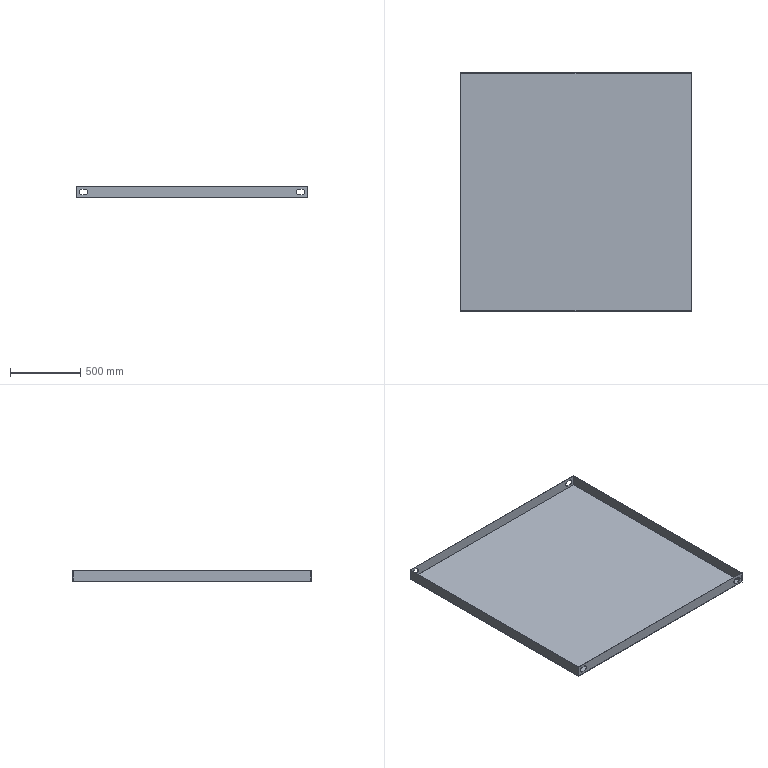Part | SolidWorks | features Extrusion 1, ICE 1, Shell 1 | 1 solid | 27 faces | box 1650 x 1700 x 80 mm | volume 7628292 mm3 | plane 19 | cylinder 8 | commonest cylinder face diameters 40 x8
STEP:
#1=CARTESIAN_POINT('',(825.,-850.,0.));
#2=VERTEX_POINT('',#1);
#3=CARTESIAN_POINT('',(825.,850.,0.));
#4=VERTEX_POINT('',#3);
#5=CARTESIAN_POINT('',(825.,850.,0.));
#6=DIRECTION('',(0.,1.,0.));
#7=VECTOR('',#6,1000.);
#8=LINE('',#5,#7);
#9=EDGE_CURVE('',#2,#4,#8,.T.);
#10=ORIENTED_EDGE('',*,*,#9,.T.);
#11=CARTESIAN_POINT('',(825.,850.,80.));
#12=VERTEX_POINT('',#11);
#13=CARTESIAN_POINT('',(825.,850.,80.));
#14=DIRECTION('',(0.,0.,-1.));
#15=VECTOR('',#14,1000.);
#16=LINE('',#13,#15);
#17=EDGE_CURVE('',#12,#4,#16,.T.);
#18=ORIENTED_EDGE('',*,*,#17,.F.);
#19=CARTESIAN_POINT('',(825.,-850.,80.));
#20=VERTEX_POINT('',#19);
#21=CARTESIAN_POINT('',(825.,850.,80.));
#22=DIRECTION('',(0.,1.,0.));
#23=VECTOR('',#22,1000.);
#24=LINE('',#21,#23);
#25=EDGE_CURVE('',#20,#12,#24,.T.);
#26=ORIENTED_EDGE('',*,*,#25,.F.);
#27=CARTESIAN_POINT('',(825.,-850.,80.));
#28=DIRECTION('',(0.,0.,-1.));
#29=VECTOR('',#28,1000.);
#30=LINE('',#27,#29);
#31=EDGE_CURVE('',#20,#2,#30,.T.);
#32=ORIENTED_EDGE('',*,*,#31,.T.);
#33=EDGE_LOOP('',(#10,#18,#26,#32));
#34=FACE_OUTER_BOUND('',#33,.T.);
#35=CARTESIAN_POINT('',(825.,850.,80.));
#36=DIRECTION('',(-1.,0.,0.));
#37=DIRECTION('',(0.,-1.,0.));
#38=AXIS2_PLACEMENT_3D('',#35,#36,#37);
#39=PLANE('',#38);
#40=ADVANCED_FACE('',(#34),#39,.F.);
#41=CARTESIAN_POINT('',(-765.,850.,60.));
#42=VERTEX_POINT('',#41);
#43=CARTESIAN_POINT('',(-785.,850.,60.));
#44=VERTEX_POINT('',#43);
#45=CARTESIAN_POINT('',(-785.,850.,60.));
#46=DIRECTION('',(-1.,0.,0.));
#47=VECTOR('',#46,1000.);
#48=LINE('',#45,#47);
#49=EDGE_CURVE('',#42,#44,#48,.T.);
#50=ORIENTED_EDGE('',*,*,#49,.T.);
#51=CARTESIAN_POINT('',(-785.,850.,20.));
#52=VERTEX_POINT('',#51);
#53=CARTESIAN_POINT('',(-785.,850.,40.));
#54=DIRECTION('',(0.,-1.,0.));
#55=DIRECTION('',(0.,0.,-1.));
#56=AXIS2_PLACEMENT_3D('',#53,#54,#55);
#57=CIRCLE('',#56,20.);
#58=EDGE_CURVE('',#44,#52,#57,.T.);
#59=ORIENTED_EDGE('',*,*,#58,.T.);
#60=CARTESIAN_POINT('',(-765.,850.,20.));
#61=VERTEX_POINT('',#60);
#62=CARTESIAN_POINT('',(-785.,850.,20.));
#63=DIRECTION('',(1.,0.,0.));
#64=VECTOR('',#63,1000.);
#65=LINE('',#62,#64);
#66=EDGE_CURVE('',#52,#61,#65,.T.);
#67=ORIENTED_EDGE('',*,*,#66,.T.);
#68=CARTESIAN_POINT('',(-765.,850.,40.));
#69=DIRECTION('',(0.,-1.,0.));
#70=DIRECTION('',(0.,0.,-1.));
#71=AXIS2_PLACEMENT_3D('',#68,#69,#70);
#72=CIRCLE('',#71,20.);
#73=EDGE_CURVE('',#61,#42,#72,.T.);
#74=ORIENTED_EDGE('',*,*,#73,.T.);
#75=EDGE_LOOP('',(#50,#59,#67,#74));
#76=FACE_BOUND('',#75,.T.);
#77=CARTESIAN_POINT('',(765.,850.,20.));
#78=VERTEX_POINT('',#77);
#79=CARTESIAN_POINT('',(785.,850.,20.));
#80=VERTEX_POINT('',#79);
#81=CARTESIAN_POINT('',(785.,850.,20.));
#82=DIRECTION('',(1.,0.,0.));
#83=VECTOR('',#82,1000.);
#84=LINE('',#81,#83);
#85=EDGE_CURVE('',#78,#80,#84,.T.);
#86=ORIENTED_EDGE('',*,*,#85,.T.);
#87=CARTESIAN_POINT('',(785.,850.,60.));
#88=VERTEX_POINT('',#87);
#89=CARTESIAN_POINT('',(785.,850.,40.));
#90=DIRECTION('',(0.,-1.,0.));
#91=DIRECTION('',(0.,0.,1.));
#92=AXIS2_PLACEMENT_3D('',#89,#90,#91);
#93=CIRCLE('',#92,20.);
#94=EDGE_CURVE('',#80,#88,#93,.T.);
#95=ORIENTED_EDGE('',*,*,#94,.T.);
#96=CARTESIAN_POINT('',(765.,850.,60.));
#97=VERTEX_POINT('',#96);
#98=CARTESIAN_POINT('',(785.,850.,60.));
#99=DIRECTION('',(-1.,0.,0.));
#100=VECTOR('',#99,1000.);
#101=LINE('',#98,#100);
#102=EDGE_CURVE('',#88,#97,#101,.T.);
#103=ORIENTED_EDGE('',*,*,#102,.T.);
#104=CARTESIAN_POINT('',(765.,850.,40.));
#105=DIRECTION('',(0.,-1.,0.));
#106=DIRECTION('',(0.,0.,1.));
#107=AXIS2_PLACEMENT_3D('',#104,#105,#106);
#108=CIRCLE('',#107,20.);
#109=EDGE_CURVE('',#97,#78,#108,.T.);
#110=ORIENTED_EDGE('',*,*,#109,.T.);
#111=EDGE_LOOP('',(#86,#95,#103,#110));
#112=FACE_BOUND('',#111,.T.);
#113=CARTESIAN_POINT('',(-825.,850.,0.));
#114=VERTEX_POINT('',#113);
#115=CARTESIAN_POINT('',(-825.,850.,0.));
#116=DIRECTION('',(-1.,0.,0.));
#117=VECTOR('',#116,1000.);
#118=LINE('',#115,#117);
#119=EDGE_CURVE('',#4,#114,#118,.T.);
#120=ORIENTED_EDGE('',*,*,#119,.T.);
#121=CARTESIAN_POINT('',(-825.,850.,80.));
#122=VERTEX_POINT('',#121);
#123=CARTESIAN_POINT('',(-825.,850.,80.));
#124=DIRECTION('',(0.,0.,-1.));
#125=VECTOR('',#124,1000.);
#126=LINE('',#123,#125);
#127=EDGE_CURVE('',#122,#114,#126,.T.);
#128=ORIENTED_EDGE('',*,*,#127,.F.);
#129=CARTESIAN_POINT('',(-825.,850.,80.));
#130=DIRECTION('',(-1.,0.,0.));
#131=VECTOR('',#130,1000.);
#132=LINE('',#129,#131);
#133=EDGE_CURVE('',#12,#122,#132,.T.);
#134=ORIENTED_EDGE('',*,*,#133,.F.);
#135=ORIENTED_EDGE('',*,*,#17,.T.);
#136=EDGE_LOOP('',(#120,#128,#134,#135));
#137=FACE_OUTER_BOUND('',#136,.T.);
#138=CARTESIAN_POINT('',(-825.,850.,80.));
#139=DIRECTION('',(0.,-1.,0.));
#140=DIRECTION('',(0.,0.,-1.));
#141=AXIS2_PLACEMENT_3D('',#138,#139,#140);
#142=PLANE('',#141);
#143=ADVANCED_FACE('',(#76,#112,#137),#142,.F.);
#144=CARTESIAN_POINT('',(-825.,-850.,0.));
#145=VERTEX_POINT('',#144);
#146=CARTESIAN_POINT('',(-825.,850.,0.));
#147=DIRECTION('',(0.,-1.,0.));
#148=VECTOR('',#147,1000.);
#149=LINE('',#146,#148);
#150=EDGE_CURVE('',#114,#145,#149,.T.);
#151=ORIENTED_EDGE('',*,*,#150,.T.);
#152=CARTESIAN_POINT('',(-825.,-850.,80.));
#153=VERTEX_POINT('',#152);
#154=CARTESIAN_POINT('',(-825.,-850.,80.));
#155=DIRECTION('',(0.,0.,-1.));
#156=VECTOR('',#155,1000.);
#157=LINE('',#154,#156);
#158=EDGE_CURVE('',#153,#145,#157,.T.);
#159=ORIENTED_EDGE('',*,*,#158,.F.);
#160=CARTESIAN_POINT('',(-825.,850.,80.));
#161=DIRECTION('',(0.,-1.,0.));
#162=VECTOR('',#161,1000.);
#163=LINE('',#160,#162);
#164=EDGE_CURVE('',#122,#153,#163,.T.);
#165=ORIENTED_EDGE('',*,*,#164,.F.);
#166=ORIENTED_EDGE('',*,*,#127,.T.);
#167=EDGE_LOOP('',(#151,#159,#165,#166));
#168=FACE_OUTER_BOUND('',#167,.T.);
#169=CARTESIAN_POINT('',(-825.,850.,80.));
#170=DIRECTION('',(1.,0.,0.));
#171=DIRECTION('',(0.,1.,0.));
#172=AXIS2_PLACEMENT_3D('',#169,#170,#171);
#173=PLANE('',#172);
#174=ADVANCED_FACE('',(#168),#173,.F.);
#175=CARTESIAN_POINT('',(-785.,-850.,20.));
#176=VERTEX_POINT('',#175);
#177=CARTESIAN_POINT('',(-765.,-850.,20.));
#178=VERTEX_POINT('',#177);
#179=CARTESIAN_POINT('',(-785.,-850.,20.));
#180=DIRECTION('',(1.,0.,0.));
#181=VECTOR('',#180,1000.);
#182=LINE('',#179,#181);
#183=EDGE_CURVE('',#176,#178,#182,.T.);
#184=ORIENTED_EDGE('',*,*,#183,.F.);
#185=CARTESIAN_POINT('',(-785.,-850.,60.));
#186=VERTEX_POINT('',#185);
#187=CARTESIAN_POINT('',(-785.,-850.,40.));
#188=DIRECTION('',(0.,-1.,0.));
#189=DIRECTION('',(0.,0.,-1.));
#190=AXIS2_PLACEMENT_3D('',#187,#188,#189);
#191=CIRCLE('',#190,20.);
#192=EDGE_CURVE('',#186,#176,#191,.T.);
#193=ORIENTED_EDGE('',*,*,#192,.F.);
#194=CARTESIAN_POINT('',(-765.,-850.,60.));
#195=VERTEX_POINT('',#194);
#196=CARTESIAN_POINT('',(-785.,-850.,60.));
#197=DIRECTION('',(-1.,0.,0.));
#198=VECTOR('',#197,1000.);
#199=LINE('',#196,#198);
#200=EDGE_CURVE('',#195,#186,#199,.T.);
#201=ORIENTED_EDGE('',*,*,#200,.F.);
#202=CARTESIAN_POINT('',(-765.,-850.,40.));
#203=DIRECTION('',(0.,-1.,0.));
#204=DIRECTION('',(0.,0.,-1.));
#205=AXIS2_PLACEMENT_3D('',#202,#203,#204);
#206=CIRCLE('',#205,20.);
#207=EDGE_CURVE('',#178,#195,#206,.T.);
#208=ORIENTED_EDGE('',*,*,#207,.F.);
#209=EDGE_LOOP('',(#184,#193,#201,#208));
#210=FACE_BOUND('',#209,.T.);
#211=CARTESIAN_POINT('',(785.,-850.,60.));
#212=VERTEX_POINT('',#211);
#213=CARTESIAN_POINT('',(765.,-850.,60.));
#214=VERTEX_POINT('',#213);
#215=CARTESIAN_POINT('',(785.,-850.,60.));
#216=DIRECTION('',(-1.,0.,0.));
#217=VECTOR('',#216,1000.);
#218=LINE('',#215,#217);
#219=EDGE_CURVE('',#212,#214,#218,.T.);
#220=ORIENTED_EDGE('',*,*,#219,.F.);
#221=CARTESIAN_POINT('',(785.,-850.,20.));
#222=VERTEX_POINT('',#221);
#223=CARTESIAN_POINT('',(785.,-850.,40.));
#224=DIRECTION('',(0.,-1.,0.));
#225=DIRECTION('',(0.,0.,1.));
#226=AXIS2_PLACEMENT_3D('',#223,#224,#225);
#227=CIRCLE('',#226,20.);
#228=EDGE_CURVE('',#222,#212,#227,.T.);
#229=ORIENTED_EDGE('',*,*,#228,.F.);
#230=CARTESIAN_POINT('',(765.,-850.,20.));
#231=VERTEX_POINT('',#230);
#232=CARTESIAN_POINT('',(785.,-850.,20.));
#233=DIRECTION('',(1.,0.,0.));
#234=VECTOR('',#233,1000.);
#235=LINE('',#232,#234);
#236=EDGE_CURVE('',#231,#222,#235,.T.);
#237=ORIENTED_EDGE('',*,*,#236,.F.);
#238=CARTESIAN_POINT('',(765.,-850.,40.));
#239=DIRECTION('',(0.,-1.,0.));
#240=DIRECTION('',(0.,0.,1.));
#241=AXIS2_PLACEMENT_3D('',#238,#239,#240);
#242=CIRCLE('',#241,20.);
#243=EDGE_CURVE('',#214,#231,#242,.T.);
#244=ORIENTED_EDGE('',*,*,#243,.F.);
#245=EDGE_LOOP('',(#220,#229,#237,#244));
#246=FACE_BOUND('',#245,.T.);
#247=CARTESIAN_POINT('',(-825.,-850.,0.));
#248=DIRECTION('',(1.,0.,0.));
#249=VECTOR('',#248,1000.);
#250=LINE('',#247,#249);
#251=EDGE_CURVE('',#145,#2,#250,.T.);
#252=ORIENTED_EDGE('',*,*,#251,.T.);
#253=ORIENTED_EDGE('',*,*,#31,.F.);
#254=CARTESIAN_POINT('',(-825.,-850.,80.));
#255=DIRECTION('',(1.,0.,0.));
#256=VECTOR('',#255,1000.);
#257=LINE('',#254,#256);
#258=EDGE_CURVE('',#153,#20,#257,.T.);
#259=ORIENTED_EDGE('',*,*,#258,.F.);
#260=ORIENTED_EDGE('',*,*,#158,.T.);
#261=EDGE_LOOP('',(#252,#253,#259,#260));
#262=FACE_OUTER_BOUND('',#261,.T.);
#263=CARTESIAN_POINT('',(-825.,-850.,80.));
#264=DIRECTION('',(0.,1.,0.));
#265=DIRECTION('',(0.,0.,1.));
#266=AXIS2_PLACEMENT_3D('',#263,#264,#265);
#267=PLANE('',#266);
#268=ADVANCED_FACE('',(#210,#246,#262),#267,.F.);
#269=CARTESIAN_POINT('',(822.7,-847.7,80.));
#270=VERTEX_POINT('',#269);
#271=CARTESIAN_POINT('',(822.7,847.7,80.));
#272=VERTEX_POINT('',#271);
#273=CARTESIAN_POINT('',(822.7,850.,80.));
#274=DIRECTION('',(0.,1.,0.));
#275=VECTOR('',#274,1000.);
#276=LINE('',#273,#275);
#277=EDGE_CURVE('',#270,#272,#276,.T.);
#278=ORIENTED_EDGE('',*,*,#277,.F.);
#279=CARTESIAN_POINT('',(-822.7,-847.7,80.));
#280=VERTEX_POINT('',#279);
#281=CARTESIAN_POINT('',(-825.,-847.7,80.));
#282=DIRECTION('',(1.,0.,0.));
#283=VECTOR('',#282,1000.);
#284=LINE('',#281,#283);
#285=EDGE_CURVE('',#280,#270,#284,.T.);
#286=ORIENTED_EDGE('',*,*,#285,.F.);
#287=CARTESIAN_POINT('',(-822.7,847.7,80.));
#288=VERTEX_POINT('',#287);
#289=CARTESIAN_POINT('',(-822.7,850.,80.));
#290=DIRECTION('',(0.,-1.,0.));
#291=VECTOR('',#290,1000.);
#292=LINE('',#289,#291);
#293=EDGE_CURVE('',#288,#280,#292,.T.);
#294=ORIENTED_EDGE('',*,*,#293,.F.);
#295=CARTESIAN_POINT('',(-825.,847.7,80.));
#296=DIRECTION('',(-1.,0.,0.));
#297=VECTOR('',#296,1000.);
#298=LINE('',#295,#297);
#299=EDGE_CURVE('',#272,#288,#298,.T.);
#300=ORIENTED_EDGE('',*,*,#299,.F.);
#301=EDGE_LOOP('',(#278,#286,#294,#300));
#302=FACE_BOUND('',#301,.T.);
#303=ORIENTED_EDGE('',*,*,#25,.T.);
#304=ORIENTED_EDGE('',*,*,#133,.T.);
#305=ORIENTED_EDGE('',*,*,#164,.T.);
#306=ORIENTED_EDGE('',*,*,#258,.T.);
#307=EDGE_LOOP('',(#303,#304,#305,#306));
#308=FACE_OUTER_BOUND('',#307,.T.);
#309=CARTESIAN_POINT('',(0.,0.,80.));
#310=DIRECTION('',(0.,0.,1.));
#311=DIRECTION('',(1.,0.,0.));
#312=AXIS2_PLACEMENT_3D('',#309,#310,#311);
#313=PLANE('',#312);
#314=ADVANCED_FACE('',(#302,#308),#313,.T.);
#315=ORIENTED_EDGE('',*,*,#9,.F.);
#316=ORIENTED_EDGE('',*,*,#251,.F.);
#317=ORIENTED_EDGE('',*,*,#150,.F.);
#318=ORIENTED_EDGE('',*,*,#119,.F.);
#319=EDGE_LOOP('',(#315,#316,#317,#318));
#320=FACE_OUTER_BOUND('',#319,.T.);
#321=CARTESIAN_POINT('',(0.,0.,0.));
#322=DIRECTION('',(0.,0.,1.));
#323=DIRECTION('',(1.,0.,0.));
#324=AXIS2_PLACEMENT_3D('',#321,#322,#323);
#325=PLANE('',#324);
#326=ADVANCED_FACE('',(#320),#325,.F.);
#327=CARTESIAN_POINT('',(822.7,-847.7,2.3));
#328=VERTEX_POINT('',#327);
#329=CARTESIAN_POINT('',(822.7,847.7,2.3));
#330=VERTEX_POINT('',#329);
#331=CARTESIAN_POINT('',(822.7,850.,2.3));
#332=DIRECTION('',(0.,1.,0.));
#333=VECTOR('',#332,1000.);
#334=LINE('',#331,#333);
#335=EDGE_CURVE('',#328,#330,#334,.T.);
#336=ORIENTED_EDGE('',*,*,#335,.F.);
#337=CARTESIAN_POINT('',(822.7,-847.7,80.));
#338=DIRECTION('',(0.,0.,-1.));
#339=VECTOR('',#338,1000.);
#340=LINE('',#337,#339);
#341=EDGE_CURVE('',#270,#328,#340,.T.);
#342=ORIENTED_EDGE('',*,*,#341,.F.);
#343=ORIENTED_EDGE('',*,*,#277,.T.);
#344=CARTESIAN_POINT('',(822.7,847.7,80.));
#345=DIRECTION('',(0.,0.,-1.));
#346=VECTOR('',#345,1000.);
#347=LINE('',#344,#346);
#348=EDGE_CURVE('',#272,#330,#347,.T.);
#349=ORIENTED_EDGE('',*,*,#348,.T.);
#350=EDGE_LOOP('',(#336,#342,#343,#349));
#351=FACE_OUTER_BOUND('',#350,.T.);
#352=CARTESIAN_POINT('',(822.7,850.,80.));
#353=DIRECTION('',(-1.,0.,0.));
#354=DIRECTION('',(0.,-1.,0.));
#355=AXIS2_PLACEMENT_3D('',#352,#353,#354);
#356=PLANE('',#355);
#357=ADVANCED_FACE('',(#351),#356,.T.);
#358=CARTESIAN_POINT('',(-785.,847.7,60.));
#359=VERTEX_POINT('',#358);
#360=CARTESIAN_POINT('',(-785.,847.7,20.));
#361=VERTEX_POINT('',#360);
#362=CARTESIAN_POINT('',(-785.,847.7,40.));
#363=DIRECTION('',(0.,-1.,0.));
#364=DIRECTION('',(0.,0.,-1.));
#365=AXIS2_PLACEMENT_3D('',#362,#363,#364);
#366=CIRCLE('',#365,20.);
#367=EDGE_CURVE('',#359,#361,#366,.T.);
#368=ORIENTED_EDGE('',*,*,#367,.F.);
#369=CARTESIAN_POINT('',(-765.,847.7,60.));
#370=VERTEX_POINT('',#369);
#371=CARTESIAN_POINT('',(-825.,847.7,60.));
#372=DIRECTION('',(-1.,0.,0.));
#373=VECTOR('',#372,1000.);
#374=LINE('',#371,#373);
#375=EDGE_CURVE('',#370,#359,#374,.T.);
#376=ORIENTED_EDGE('',*,*,#375,.F.);
#377=CARTESIAN_POINT('',(-765.,847.7,20.));
#378=VERTEX_POINT('',#377);
#379=CARTESIAN_POINT('',(-765.,847.7,40.));
#380=DIRECTION('',(0.,-1.,0.));
#381=DIRECTION('',(0.,0.,-1.));
#382=AXIS2_PLACEMENT_3D('',#379,#380,#381);
#383=CIRCLE('',#382,20.);
#384=EDGE_CURVE('',#378,#370,#383,.T.);
#385=ORIENTED_EDGE('',*,*,#384,.F.);
#386=CARTESIAN_POINT('',(-825.,847.7,20.));
#387=DIRECTION('',(1.,0.,0.));
#388=VECTOR('',#387,1000.);
#389=LINE('',#386,#388);
#390=EDGE_CURVE('',#361,#378,#389,.T.);
#391=ORIENTED_EDGE('',*,*,#390,.F.);
#392=EDGE_LOOP('',(#368,#376,#385,#391));
#393=FACE_BOUND('',#392,.T.);
#394=CARTESIAN_POINT('',(785.,847.7,20.));
#395=VERTEX_POINT('',#394);
#396=CARTESIAN_POINT('',(785.,847.7,60.));
#397=VERTEX_POINT('',#396);
#398=CARTESIAN_POINT('',(785.,847.7,40.));
#399=DIRECTION('',(0.,-1.,0.));
#400=DIRECTION('',(0.,0.,-1.));
#401=AXIS2_PLACEMENT_3D('',#398,#399,#400);
#402=CIRCLE('',#401,20.);
#403=EDGE_CURVE('',#395,#397,#402,.T.);
#404=ORIENTED_EDGE('',*,*,#403,.F.);
#405=CARTESIAN_POINT('',(765.,847.7,20.));
#406=VERTEX_POINT('',#405);
#407=CARTESIAN_POINT('',(-825.,847.7,20.));
#408=DIRECTION('',(1.,0.,0.));
#409=VECTOR('',#408,1000.);
#410=LINE('',#407,#409);
#411=EDGE_CURVE('',#406,#395,#410,.T.);
#412=ORIENTED_EDGE('',*,*,#411,.F.);
#413=CARTESIAN_POINT('',(765.,847.7,60.));
#414=VERTEX_POINT('',#413);
#415=CARTESIAN_POINT('',(765.,847.7,40.));
#416=DIRECTION('',(0.,-1.,0.));
#417=DIRECTION('',(0.,0.,-1.));
#418=AXIS2_PLACEMENT_3D('',#415,#416,#417);
#419=CIRCLE('',#418,20.);
#420=EDGE_CURVE('',#414,#406,#419,.T.);
#421=ORIENTED_EDGE('',*,*,#420,.F.);
#422=CARTESIAN_POINT('',(-825.,847.7,60.));
#423=DIRECTION('',(-1.,0.,0.));
#424=VECTOR('',#423,1000.);
#425=LINE('',#422,#424);
#426=EDGE_CURVE('',#397,#414,#425,.T.);
#427=ORIENTED_EDGE('',*,*,#426,.F.);
#428=EDGE_LOOP('',(#404,#412,#421,#427));
#429=FACE_BOUND('',#428,.T.);
#430=CARTESIAN_POINT('',(-822.7,847.7,2.3));
#431=VERTEX_POINT('',#430);
#432=CARTESIAN_POINT('',(-825.,847.7,2.3));
#433=DIRECTION('',(-1.,0.,0.));
#434=VECTOR('',#433,1000.);
#435=LINE('',#432,#434);
#436=EDGE_CURVE('',#330,#431,#435,.T.);
#437=ORIENTED_EDGE('',*,*,#436,.F.);
#438=ORIENTED_EDGE('',*,*,#348,.F.);
#439=ORIENTED_EDGE('',*,*,#299,.T.);
#440=CARTESIAN_POINT('',(-822.7,847.7,80.));
#441=DIRECTION('',(0.,0.,-1.));
#442=VECTOR('',#441,1000.);
#443=LINE('',#440,#442);
#444=EDGE_CURVE('',#288,#431,#443,.T.);
#445=ORIENTED_EDGE('',*,*,#444,.T.);
#446=EDGE_LOOP('',(#437,#438,#439,#445));
#447=FACE_OUTER_BOUND('',#446,.T.);
#448=CARTESIAN_POINT('',(-825.,847.7,80.));
#449=DIRECTION('',(0.,-1.,0.));
#450=DIRECTION('',(0.,0.,-1.));
#451=AXIS2_PLACEMENT_3D('',#448,#449,#450);
#452=PLANE('',#451);
#453=ADVANCED_FACE('',(#393,#429,#447),#452,.T.);
#454=CARTESIAN_POINT('',(-822.7,-847.7,2.3));
#455=VERTEX_POINT('',#454);
#456=CARTESIAN_POINT('',(-822.7,850.,2.3));
#457=DIRECTION('',(0.,-1.,0.));
#458=VECTOR('',#457,1000.);
#459=LINE('',#456,#458);
#460=EDGE_CURVE('',#431,#455,#459,.T.);
#461=ORIENTED_EDGE('',*,*,#460,.F.);
#462=ORIENTED_EDGE('',*,*,#444,.F.);
#463=ORIENTED_EDGE('',*,*,#293,.T.);
#464=CARTESIAN_POINT('',(-822.7,-847.7,80.));
#465=DIRECTION('',(0.,0.,-1.));
#466=VECTOR('',#465,1000.);
#467=LINE('',#464,#466);
#468=EDGE_CURVE('',#280,#455,#467,.T.);
#469=ORIENTED_EDGE('',*,*,#468,.T.);
#470=EDGE_LOOP('',(#461,#462,#463,#469));
#471=FACE_OUTER_BOUND('',#470,.T.);
#472=CARTESIAN_POINT('',(-822.7,850.,80.));
#473=DIRECTION('',(1.,0.,0.));
#474=DIRECTION('',(0.,1.,0.));
#475=AXIS2_PLACEMENT_3D('',#472,#473,#474);
#476=PLANE('',#475);
#477=ADVANCED_FACE('',(#471),#476,.T.);
#478=CARTESIAN_POINT('',(-785.,-847.7,20.));
#479=VERTEX_POINT('',#478);
#480=CARTESIAN_POINT('',(-785.,-847.7,60.));
#481=VERTEX_POINT('',#480);
#482=CARTESIAN_POINT('',(-785.,-847.7,40.));
#483=DIRECTION('',(0.,1.,0.));
#484=DIRECTION('',(0.,0.,1.));
#485=AXIS2_PLACEMENT_3D('',#482,#483,#484);
#486=CIRCLE('',#485,20.);
#487=EDGE_CURVE('',#479,#481,#486,.T.);
#488=ORIENTED_EDGE('',*,*,#487,.F.);
#489=CARTESIAN_POINT('',(-765.,-847.7,20.));
#490=VERTEX_POINT('',#489);
#491=CARTESIAN_POINT('',(-825.,-847.7,20.));
#492=DIRECTION('',(-1.,0.,0.));
#493=VECTOR('',#492,1000.);
#494=LINE('',#491,#493);
#495=EDGE_CURVE('',#490,#479,#494,.T.);
#496=ORIENTED_EDGE('',*,*,#495,.F.);
#497=CARTESIAN_POINT('',(-765.,-847.7,60.));
#498=VERTEX_POINT('',#497);
#499=CARTESIAN_POINT('',(-765.,-847.7,40.));
#500=DIRECTION('',(0.,1.,0.));
#501=DIRECTION('',(0.,0.,1.));
#502=AXIS2_PLACEMENT_3D('',#499,#500,#501);
#503=CIRCLE('',#502,20.);
#504=EDGE_CURVE('',#498,#490,#503,.T.);
#505=ORIENTED_EDGE('',*,*,#504,.F.);
#506=CARTESIAN_POINT('',(-825.,-847.7,60.));
#507=DIRECTION('',(1.,0.,0.));
#508=VECTOR('',#507,1000.);
#509=LINE('',#506,#508);
#510=EDGE_CURVE('',#481,#498,#509,.T.);
#511=ORIENTED_EDGE('',*,*,#510,.F.);
#512=EDGE_LOOP('',(#488,#496,#505,#511));
#513=FACE_BOUND('',#512,.T.);
#514=CARTESIAN_POINT('',(785.,-847.7,60.));
#515=VERTEX_POINT('',#514);
#516=CARTESIAN_POINT('',(785.,-847.7,20.));
#517=VERTEX_POINT('',#516);
#518=CARTESIAN_POINT('',(785.,-847.7,40.));
#519=DIRECTION('',(0.,1.,0.));
#520=DIRECTION('',(0.,0.,1.));
#521=AXIS2_PLACEMENT_3D('',#518,#519,#520);
#522=CIRCLE('',#521,20.);
#523=EDGE_CURVE('',#515,#517,#522,.T.);
#524=ORIENTED_EDGE('',*,*,#523,.F.);
#525=CARTESIAN_POINT('',(765.,-847.7,60.));
#526=VERTEX_POINT('',#525);
#527=CARTESIAN_POINT('',(-825.,-847.7,60.));
#528=DIRECTION('',(1.,0.,0.));
#529=VECTOR('',#528,1000.);
#530=LINE('',#527,#529);
#531=EDGE_CURVE('',#526,#515,#530,.T.);
#532=ORIENTED_EDGE('',*,*,#531,.F.);
#533=CARTESIAN_POINT('',(765.,-847.7,20.));
#534=VERTEX_POINT('',#533);
#535=CARTESIAN_POINT('',(765.,-847.7,40.));
#536=DIRECTION('',(0.,1.,0.));
#537=DIRECTION('',(0.,0.,1.));
#538=AXIS2_PLACEMENT_3D('',#535,#536,#537);
#539=CIRCLE('',#538,20.);
#540=EDGE_CURVE('',#534,#526,#539,.T.);
#541=ORIENTED_EDGE('',*,*,#540,.F.);
#542=CARTESIAN_POINT('',(-825.,-847.7,20.));
#543=DIRECTION('',(-1.,0.,0.));
#544=VECTOR('',#543,1000.);
#545=LINE('',#542,#544);
#546=EDGE_CURVE('',#517,#534,#545,.T.);
#547=ORIENTED_EDGE('',*,*,#546,.F.);
#548=EDGE_LOOP('',(#524,#532,#541,#547));
#549=FACE_BOUND('',#548,.T.);
#550=CARTESIAN_POINT('',(-825.,-847.7,2.3));
#551=DIRECTION('',(1.,0.,0.));
#552=VECTOR('',#551,1000.);
#553=LINE('',#550,#552);
#554=EDGE_CURVE('',#455,#328,#553,.T.);
#555=ORIENTED_EDGE('',*,*,#554,.F.);
#556=ORIENTED_EDGE('',*,*,#468,.F.);
#557=ORIENTED_EDGE('',*,*,#285,.T.);
#558=ORIENTED_EDGE('',*,*,#341,.T.);
#559=EDGE_LOOP('',(#555,#556,#557,#558));
#560=FACE_OUTER_BOUND('',#559,.T.);
#561=CARTESIAN_POINT('',(-825.,-847.7,80.));
#562=DIRECTION('',(0.,1.,0.));
#563=DIRECTION('',(0.,0.,1.));
#564=AXIS2_PLACEMENT_3D('',#561,#562,#563);
#565=PLANE('',#564);
#566=ADVANCED_FACE('',(#513,#549,#560),#565,.T.);
#567=ORIENTED_EDGE('',*,*,#335,.T.);
#568=ORIENTED_EDGE('',*,*,#436,.T.);
#569=ORIENTED_EDGE('',*,*,#460,.T.);
#570=ORIENTED_EDGE('',*,*,#554,.T.);
#571=EDGE_LOOP('',(#567,#568,#569,#570));
#572=FACE_OUTER_BOUND('',#571,.T.);
#573=CARTESIAN_POINT('',(0.,0.,2.3));
#574=DIRECTION('',(0.,0.,1.));
#575=DIRECTION('',(1.,0.,0.));
#576=AXIS2_PLACEMENT_3D('',#573,#574,#575);
#577=PLANE('',#576);
#578=ADVANCED_FACE('',(#572),#577,.T.);
#579=ORIENTED_EDGE('',*,*,#531,.T.);
#580=CARTESIAN_POINT('',(785.,850.,60.));
#581=DIRECTION('',(0.,-1.,0.));
#582=VECTOR('',#581,1000.);
#583=LINE('',#580,#582);
#584=EDGE_CURVE('',#515,#212,#583,.T.);
#585=ORIENTED_EDGE('',*,*,#584,.T.);
#586=ORIENTED_EDGE('',*,*,#219,.T.);
#587=CARTESIAN_POINT('',(765.,850.,60.));
#588=DIRECTION('',(0.,-1.,0.));
#589=VECTOR('',#588,1000.);
#590=LINE('',#587,#589);
#591=EDGE_CURVE('',#526,#214,#590,.T.);
#592=ORIENTED_EDGE('',*,*,#591,.F.);
#593=EDGE_LOOP('',(#579,#585,#586,#592));
#594=FACE_OUTER_BOUND('',#593,.T.);
#595=CARTESIAN_POINT('',(785.,850.,60.));
#596=DIRECTION('',(0.,0.,1.));
#597=DIRECTION('',(1.,0.,0.));
#598=AXIS2_PLACEMENT_3D('',#595,#596,#597);
#599=PLANE('',#598);
#600=ADVANCED_FACE('',(#594),#599,.F.);
#601=ORIENTED_EDGE('',*,*,#540,.T.);
#602=ORIENTED_EDGE('',*,*,#591,.T.);
#603=ORIENTED_EDGE('',*,*,#243,.T.);
#604=CARTESIAN_POINT('',(765.,850.,20.));
#605=DIRECTION('',(0.,-1.,0.));
#606=VECTOR('',#605,1000.);
#607=LINE('',#604,#606);
#608=EDGE_CURVE('',#534,#231,#607,.T.);
#609=ORIENTED_EDGE('',*,*,#608,.F.);
#610=EDGE_LOOP('',(#601,#602,#603,#609));
#611=FACE_OUTER_BOUND('',#610,.T.);
#612=CARTESIAN_POINT('',(765.,850.,40.));
#613=DIRECTION('',(0.,-1.,0.));
#614=DIRECTION('',(0.,0.,-1.));
#615=AXIS2_PLACEMENT_3D('',#612,#613,#614);
#616=CYLINDRICAL_SURFACE('',#615,20.);
#617=ADVANCED_FACE('',(#611),#616,.F.);
#618=ORIENTED_EDGE('',*,*,#546,.T.);
#619=ORIENTED_EDGE('',*,*,#608,.T.);
#620=ORIENTED_EDGE('',*,*,#236,.T.);
#621=CARTESIAN_POINT('',(785.,850.,20.));
#622=DIRECTION('',(0.,-1.,0.));
#623=VECTOR('',#622,1000.);
#624=LINE('',#621,#623);
#625=EDGE_CURVE('',#517,#222,#624,.T.);
#626=ORIENTED_EDGE('',*,*,#625,.F.);
#627=EDGE_LOOP('',(#618,#619,#620,#626));
#628=FACE_OUTER_BOUND('',#627,.T.);
#629=CARTESIAN_POINT('',(785.,850.,20.));
#630=DIRECTION('',(0.,0.,-1.));
#631=DIRECTION('',(-1.,0.,0.));
#632=AXIS2_PLACEMENT_3D('',#629,#630,#631);
#633=PLANE('',#632);
#634=ADVANCED_FACE('',(#628),#633,.F.);
#635=ORIENTED_EDGE('',*,*,#523,.T.);
#636=ORIENTED_EDGE('',*,*,#625,.T.);
#637=ORIENTED_EDGE('',*,*,#228,.T.);
#638=ORIENTED_EDGE('',*,*,#584,.F.);
#639=EDGE_LOOP('',(#635,#636,#637,#638));
#640=FACE_OUTER_BOUND('',#639,.T.);
#641=CARTESIAN_POINT('',(785.,850.,40.));
#642=DIRECTION('',(0.,-1.,0.));
#643=DIRECTION('',(0.,0.,-1.));
#644=AXIS2_PLACEMENT_3D('',#641,#642,#643);
#645=CYLINDRICAL_SURFACE('',#644,20.);
#646=ADVANCED_FACE('',(#640),#645,.F.);
#647=ORIENTED_EDGE('',*,*,#495,.T.);
#648=CARTESIAN_POINT('',(-785.,850.,20.));
#649=DIRECTION('',(0.,-1.,0.));
#650=VECTOR('',#649,1000.);
#651=LINE('',#648,#650);
#652=EDGE_CURVE('',#479,#176,#651,.T.);
#653=ORIENTED_EDGE('',*,*,#652,.T.);
#654=ORIENTED_EDGE('',*,*,#183,.T.);
#655=CARTESIAN_POINT('',(-765.,850.,20.));
#656=DIRECTION('',(0.,-1.,0.));
#657=VECTOR('',#656,1000.);
#658=LINE('',#655,#657);
#659=EDGE_CURVE('',#490,#178,#658,.T.);
#660=ORIENTED_EDGE('',*,*,#659,.F.);
#661=EDGE_LOOP('',(#647,#653,#654,#660));
#662=FACE_OUTER_BOUND('',#661,.T.);
#663=CARTESIAN_POINT('',(-785.,850.,20.));
#664=DIRECTION('',(0.,0.,-1.));
#665=DIRECTION('',(-1.,0.,0.));
#666=AXIS2_PLACEMENT_3D('',#663,#664,#665);
#667=PLANE('',#666);
#668=ADVANCED_FACE('',(#662),#667,.F.);
#669=ORIENTED_EDGE('',*,*,#504,.T.);
#670=ORIENTED_EDGE('',*,*,#659,.T.);
#671=ORIENTED_EDGE('',*,*,#207,.T.);
#672=CARTESIAN_POINT('',(-765.,850.,60.));
#673=DIRECTION('',(0.,-1.,0.));
#674=VECTOR('',#673,1000.);
#675=LINE('',#672,#674);
#676=EDGE_CURVE('',#498,#195,#675,.T.);
#677=ORIENTED_EDGE('',*,*,#676,.F.);
#678=EDGE_LOOP('',(#669,#670,#671,#677));
#679=FACE_OUTER_BOUND('',#678,.T.);
#680=CARTESIAN_POINT('',(-765.,850.,40.));
#681=DIRECTION('',(0.,-1.,0.));
#682=DIRECTION('',(0.,0.,-1.));
#683=AXIS2_PLACEMENT_3D('',#680,#681,#682);
#684=CYLINDRICAL_SURFACE('',#683,20.);
#685=ADVANCED_FACE('',(#679),#684,.F.);
#686=ORIENTED_EDGE('',*,*,#510,.T.);
#687=ORIENTED_EDGE('',*,*,#676,.T.);
#688=ORIENTED_EDGE('',*,*,#200,.T.);
#689=CARTESIAN_POINT('',(-785.,850.,60.));
#690=DIRECTION('',(0.,-1.,0.));
#691=VECTOR('',#690,1000.);
#692=LINE('',#689,#691);
#693=EDGE_CURVE('',#481,#186,#692,.T.);
#694=ORIENTED_EDGE('',*,*,#693,.F.);
#695=EDGE_LOOP('',(#686,#687,#688,#694));
#696=FACE_OUTER_BOUND('',#695,.T.);
#697=CARTESIAN_POINT('',(-785.,850.,60.));
#698=DIRECTION('',(0.,0.,1.));
#699=DIRECTION('',(1.,0.,0.));
#700=AXIS2_PLACEMENT_3D('',#697,#698,#699);
#701=PLANE('',#700);
#702=ADVANCED_FACE('',(#696),#701,.F.);
#703=ORIENTED_EDGE('',*,*,#487,.T.);
#704=ORIENTED_EDGE('',*,*,#693,.T.);
#705=ORIENTED_EDGE('',*,*,#192,.T.);
#706=ORIENTED_EDGE('',*,*,#652,.F.);
#707=EDGE_LOOP('',(#703,#704,#705,#706));
#708=FACE_OUTER_BOUND('',#707,.T.);
#709=CARTESIAN_POINT('',(-785.,850.,40.));
#710=DIRECTION('',(0.,-1.,0.));
#711=DIRECTION('',(0.,0.,-1.));
#712=AXIS2_PLACEMENT_3D('',#709,#710,#711);
#713=CYLINDRICAL_SURFACE('',#712,20.);
#714=ADVANCED_FACE('',(#708),#713,.F.);
#715=ORIENTED_EDGE('',*,*,#403,.T.);
#716=CARTESIAN_POINT('',(785.,850.,60.));
#717=DIRECTION('',(0.,-1.,0.));
#718=VECTOR('',#717,1000.);
#719=LINE('',#716,#718);
#720=EDGE_CURVE('',#88,#397,#719,.T.);
#721=ORIENTED_EDGE('',*,*,#720,.F.);
#722=ORIENTED_EDGE('',*,*,#94,.F.);
#723=CARTESIAN_POINT('',(785.,850.,20.));
#724=DIRECTION('',(0.,-1.,0.));
#725=VECTOR('',#724,1000.);
#726=LINE('',#723,#725);
#727=EDGE_CURVE('',#80,#395,#726,.T.);
#728=ORIENTED_EDGE('',*,*,#727,.T.);
#729=EDGE_LOOP('',(#715,#721,#722,#728));
#730=FACE_OUTER_BOUND('',#729,.T.);
#731=CARTESIAN_POINT('',(785.,850.,40.));
#732=DIRECTION('',(0.,-1.,0.));
#733=DIRECTION('',(0.,0.,-1.));
#734=AXIS2_PLACEMENT_3D('',#731,#732,#733);
#735=CYLINDRICAL_SURFACE('',#734,20.);
#736=ADVANCED_FACE('',(#730),#735,.F.);
#737=ORIENTED_EDGE('',*,*,#411,.T.);
#738=ORIENTED_EDGE('',*,*,#727,.F.);
#739=ORIENTED_EDGE('',*,*,#85,.F.);
#740=CARTESIAN_POINT('',(765.,850.,20.));
#741=DIRECTION('',(0.,-1.,0.));
#742=VECTOR('',#741,1000.);
#743=LINE('',#740,#742);
#744=EDGE_CURVE('',#78,#406,#743,.T.);
#745=ORIENTED_EDGE('',*,*,#744,.T.);
#746=EDGE_LOOP('',(#737,#738,#739,#745));
#747=FACE_OUTER_BOUND('',#746,.T.);
#748=CARTESIAN_POINT('',(785.,850.,20.));
#749=DIRECTION('',(0.,0.,-1.));
#750=DIRECTION('',(-1.,0.,0.));
#751=AXIS2_PLACEMENT_3D('',#748,#749,#750);
#752=PLANE('',#751);
#753=ADVANCED_FACE('',(#747),#752,.F.);
#754=ORIENTED_EDGE('',*,*,#420,.T.);
#755=ORIENTED_EDGE('',*,*,#744,.F.);
#756=ORIENTED_EDGE('',*,*,#109,.F.);
#757=CARTESIAN_POINT('',(765.,850.,60.));
#758=DIRECTION('',(0.,-1.,0.));
#759=VECTOR('',#758,1000.);
#760=LINE('',#757,#759);
#761=EDGE_CURVE('',#97,#414,#760,.T.);
#762=ORIENTED_EDGE('',*,*,#761,.T.);
#763=EDGE_LOOP('',(#754,#755,#756,#762));
#764=FACE_OUTER_BOUND('',#763,.T.);
#765=CARTESIAN_POINT('',(765.,850.,40.));
#766=DIRECTION('',(0.,-1.,0.));
#767=DIRECTION('',(0.,0.,-1.));
#768=AXIS2_PLACEMENT_3D('',#765,#766,#767);
#769=CYLINDRICAL_SURFACE('',#768,20.);
#770=ADVANCED_FACE('',(#764),#769,.F.);
#771=ORIENTED_EDGE('',*,*,#426,.T.);
#772=ORIENTED_EDGE('',*,*,#761,.F.);
#773=ORIENTED_EDGE('',*,*,#102,.F.);
#774=ORIENTED_EDGE('',*,*,#720,.T.);
#775=EDGE_LOOP('',(#771,#772,#773,#774));
#776=FACE_OUTER_BOUND('',#775,.T.);
#777=CARTESIAN_POINT('',(785.,850.,60.));
#778=DIRECTION('',(0.,0.,1.));
#779=DIRECTION('',(1.,0.,0.));
#780=AXIS2_PLACEMENT_3D('',#777,#778,#779);
#781=PLANE('',#780);
#782=ADVANCED_FACE('',(#776),#781,.F.);
#783=ORIENTED_EDGE('',*,*,#367,.T.);
#784=CARTESIAN_POINT('',(-785.,850.,20.));
#785=DIRECTION('',(0.,-1.,0.));
#786=VECTOR('',#785,1000.);
#787=LINE('',#784,#786);
#788=EDGE_CURVE('',#52,#361,#787,.T.);
#789=ORIENTED_EDGE('',*,*,#788,.F.);
#790=ORIENTED_EDGE('',*,*,#58,.F.);
#791=CARTESIAN_POINT('',(-785.,850.,60.));
#792=DIRECTION('',(0.,-1.,0.));
#793=VECTOR('',#792,1000.);
#794=LINE('',#791,#793);
#795=EDGE_CURVE('',#44,#359,#794,.T.);
#796=ORIENTED_EDGE('',*,*,#795,.T.);
#797=EDGE_LOOP('',(#783,#789,#790,#796));
#798=FACE_OUTER_BOUND('',#797,.T.);
#799=CARTESIAN_POINT('',(-785.,850.,40.));
#800=DIRECTION('',(0.,-1.,0.));
#801=DIRECTION('',(0.,0.,-1.));
#802=AXIS2_PLACEMENT_3D('',#799,#800,#801);
#803=CYLINDRICAL_SURFACE('',#802,20.);
#804=ADVANCED_FACE('',(#798),#803,.F.);
#805=ORIENTED_EDGE('',*,*,#375,.T.);
#806=ORIENTED_EDGE('',*,*,#795,.F.);
#807=ORIENTED_EDGE('',*,*,#49,.F.);
#808=CARTESIAN_POINT('',(-765.,850.,60.));
#809=DIRECTION('',(0.,-1.,0.));
#810=VECTOR('',#809,1000.);
#811=LINE('',#808,#810);
#812=EDGE_CURVE('',#42,#370,#811,.T.);
#813=ORIENTED_EDGE('',*,*,#812,.T.);
#814=EDGE_LOOP('',(#805,#806,#807,#813));
#815=FACE_OUTER_BOUND('',#814,.T.);
#816=CARTESIAN_POINT('',(-785.,850.,60.));
#817=DIRECTION('',(0.,0.,1.));
#818=DIRECTION('',(1.,0.,0.));
#819=AXIS2_PLACEMENT_3D('',#816,#817,#818);
#820=PLANE('',#819);
#821=ADVANCED_FACE('',(#815),#820,.F.);
#822=ORIENTED_EDGE('',*,*,#384,.T.);
#823=ORIENTED_EDGE('',*,*,#812,.F.);
#824=ORIENTED_EDGE('',*,*,#73,.F.);
#825=CARTESIAN_POINT('',(-765.,850.,20.));
#826=DIRECTION('',(0.,-1.,0.));
#827=VECTOR('',#826,1000.);
#828=LINE('',#825,#827);
#829=EDGE_CURVE('',#61,#378,#828,.T.);
#830=ORIENTED_EDGE('',*,*,#829,.T.);
#831=EDGE_LOOP('',(#822,#823,#824,#830));
#832=FACE_OUTER_BOUND('',#831,.T.);
#833=CARTESIAN_POINT('',(-765.,850.,40.));
#834=DIRECTION('',(0.,-1.,0.));
#835=DIRECTION('',(0.,0.,-1.));
#836=AXIS2_PLACEMENT_3D('',#833,#834,#835);
#837=CYLINDRICAL_SURFACE('',#836,20.);
#838=ADVANCED_FACE('',(#832),#837,.F.);
#839=ORIENTED_EDGE('',*,*,#390,.T.);
#840=ORIENTED_EDGE('',*,*,#829,.F.);
#841=ORIENTED_EDGE('',*,*,#66,.F.);
#842=ORIENTED_EDGE('',*,*,#788,.T.);
#843=EDGE_LOOP('',(#839,#840,#841,#842));
#844=FACE_OUTER_BOUND('',#843,.T.);
#845=CARTESIAN_POINT('',(-785.,850.,20.));
#846=DIRECTION('',(0.,0.,-1.));
#847=DIRECTION('',(-1.,0.,0.));
#848=AXIS2_PLACEMENT_3D('',#845,#846,#847);
#849=PLANE('',#848);
#850=ADVANCED_FACE('',(#844),#849,.F.);
#851=CLOSED_SHELL('',(#40,#143,#174,#268,#314,#326,#357,#453,#477,#566,#578,#600,#617,#634,#646,#668,#685,#702,#714,#736,#753,#770,#782,#804,#821,#838,#850));
#852=MANIFOLD_SOLID_BREP('',#851);
#853=CARTESIAN_POINT('',(0.,0.,0.));
#854=DIRECTION('',(0.,0.,1.));
#855=DIRECTION('',(1.,0.,0.));
#856=AXIS2_PLACEMENT_3D('',#853,#854,#855);
#857=(LENGTH_UNIT()NAMED_UNIT(*)SI_UNIT(.MILLI.,.METRE.));
#858=UNCERTAINTY_MEASURE_WITH_UNIT(LENGTH_MEASURE(0.00001),#857,'','');
#859=(NAMED_UNIT(*)PLANE_ANGLE_UNIT()SI_UNIT($,.RADIAN.));
#860=(NAMED_UNIT(*)SI_UNIT($,.STERADIAN.)SOLID_ANGLE_UNIT());
#861=(GEOMETRIC_REPRESENTATION_CONTEXT(3)GLOBAL_UNCERTAINTY_ASSIGNED_CONTEXT((#858))GLOBAL_UNIT_ASSIGNED_CONTEXT((#857,#859,#860))REPRESENTATION_CONTEXT('',''));
#862=ADVANCED_BREP_SHAPE_REPRESENTATION('',(#852,#856),#861);